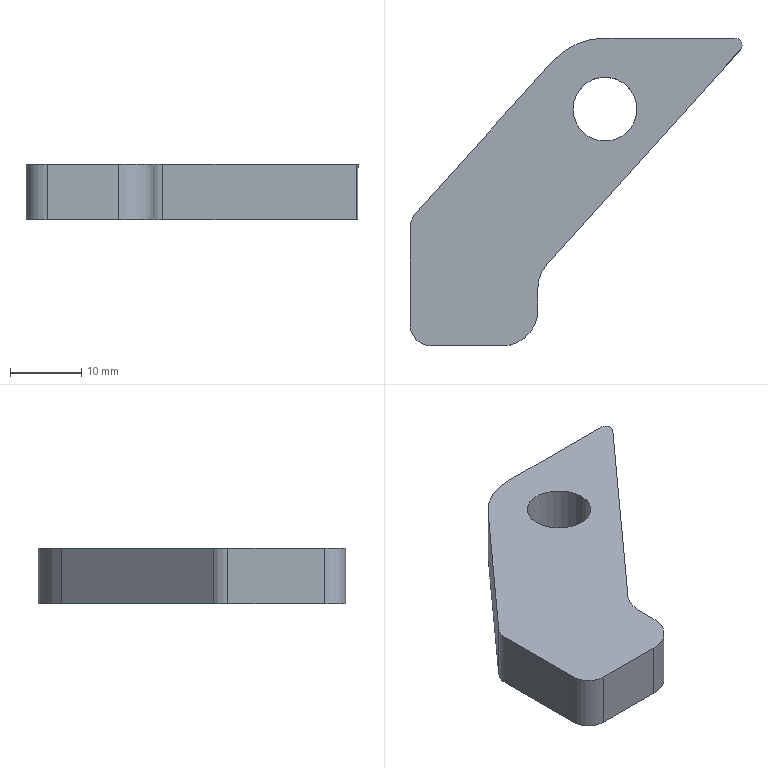Part | STEP file | 1 solid | 16 faces | box 46.755 x 43.333 x 7.8 mm | volume 7112 mm3 | cylinder 8 | plane 8 | commonest cylinder face diameters 6 x2 9 x2 10 x2 2 x1 20 x1
STEP:
#1=CARTESIAN_POINT('',(0.,0.,0.));
#2=DIRECTION('',(0.,0.,1.));
#3=DIRECTION('',(1.,0.,0.));
#4=AXIS2_PLACEMENT_3D('',#1,#2,#3);
#5=CARTESIAN_POINT('',(13.954,35.,7.8));
#6=VERTEX_POINT('',#5);
#7=CARTESIAN_POINT('',(4.954,35.,7.8));
#8=VERTEX_POINT('',#7);
#9=CARTESIAN_POINT('',(9.454,35.,7.8));
#10=DIRECTION('',(0.,0.,1.));
#11=DIRECTION('',(1.,0.,0.));
#12=AXIS2_PLACEMENT_3D('',#9,#10,#11);
#13=CIRCLE('',#12,4.5);
#14=CARTESIAN_POINT('',(9.454,35.,7.8));
#15=DIRECTION('',(0.,0.,1.));
#16=DIRECTION('',(1.,0.,0.));
#17=AXIS2_PLACEMENT_3D('',#14,#15,#16);
#18=CYLINDRICAL_SURFACE('',#17,4.5);
#19=CARTESIAN_POINT('',(0.,0.));
#20=DIRECTION('',(1.,0.));
#21=VECTOR('',#20,1.);
#22=LINE('',#19,#21);
#23=(GEOMETRIC_REPRESENTATION_CONTEXT(2)PARAMETRIC_REPRESENTATION_CONTEXT()REPRESENTATION_CONTEXT('',''));
#24=DEFINITIONAL_REPRESENTATION('',(#22),#23);
#25=PCURVE('',#18,#24);
#26=CARTESIAN_POINT('',(-15.,4.667,7.8));
#27=DIRECTION('',(0.,0.,-1.));
#28=DIRECTION('',(-1.,0.,0.));
#29=AXIS2_PLACEMENT_3D('',#26,#27,#28);
#30=PLANE('',#29);
#31=CARTESIAN_POINT('',(-28.954,30.333));
#32=CARTESIAN_POINT('',(-28.954,38.128));
#33=CARTESIAN_POINT('',(-22.204,34.23));
#34=CARTESIAN_POINT('',(-15.454,30.333));
#35=CARTESIAN_POINT('',(-22.204,26.436));
#36=CARTESIAN_POINT('',(-28.954,22.539));
#37=CARTESIAN_POINT('',(-28.954,30.333));
#38=(BOUNDED_CURVE()B_SPLINE_CURVE(2,(#31,#32,#33,#34,#35,#36,#37),.UNSPECIFIED.,.T.,.F.)B_SPLINE_CURVE_WITH_KNOTS((1,2,2,2,2,1),(-2.094,0.,2.094,4.189,6.283,8.378),.UNSPECIFIED.)CURVE()GEOMETRIC_REPRESENTATION_ITEM()RATIONAL_B_SPLINE_CURVE((1.,0.5,1.,0.5,1.,0.5,1.))REPRESENTATION_ITEM(''));
#39=(GEOMETRIC_REPRESENTATION_CONTEXT(2)PARAMETRIC_REPRESENTATION_CONTEXT()REPRESENTATION_CONTEXT('',''));
#40=DEFINITIONAL_REPRESENTATION('',(#38),#39);
#41=PCURVE('',#30,#40);
#42=SURFACE_CURVE('',#13,(#25,#41),.PCURVE_S1.);
#43=EDGE_CURVE('',#6,#8,#42,.T.);
#44=ORIENTED_EDGE('',*,*,#43,.F.);
#45=CARTESIAN_POINT('',(13.954,35.,0.));
#46=VERTEX_POINT('',#45);
#47=CARTESIAN_POINT('',(13.954,35.,7.8));
#48=DIRECTION('',(0.,0.,1.));
#49=VECTOR('',#48,1.);
#50=LINE('',#47,#49);
#51=CARTESIAN_POINT('',(0.,0.));
#52=DIRECTION('',(0.,1.));
#53=VECTOR('',#52,1.);
#54=LINE('',#51,#53);
#55=(GEOMETRIC_REPRESENTATION_CONTEXT(2)PARAMETRIC_REPRESENTATION_CONTEXT()REPRESENTATION_CONTEXT('',''));
#56=DEFINITIONAL_REPRESENTATION('',(#54),#55);
#57=PCURVE('',#18,#56);
#58=CARTESIAN_POINT('',(9.454,35.,7.8));
#59=DIRECTION('',(0.,0.,1.));
#60=DIRECTION('',(1.,0.,0.));
#61=AXIS2_PLACEMENT_3D('',#58,#59,#60);
#62=CYLINDRICAL_SURFACE('',#61,4.5);
#63=CARTESIAN_POINT('',(6.283,0.));
#64=DIRECTION('',(0.,1.));
#65=VECTOR('',#64,1.);
#66=LINE('',#63,#65);
#67=(GEOMETRIC_REPRESENTATION_CONTEXT(2)PARAMETRIC_REPRESENTATION_CONTEXT()REPRESENTATION_CONTEXT('',''));
#68=DEFINITIONAL_REPRESENTATION('',(#66),#67);
#69=PCURVE('',#62,#68);
#70=SURFACE_CURVE('',#50,(#57,#69),.PCURVE_S1.);
#71=EDGE_CURVE('',#46,#6,#70,.T.);
#72=ORIENTED_EDGE('',*,*,#71,.F.);
#73=CARTESIAN_POINT('',(4.954,35.,0.));
#74=VERTEX_POINT('',#73);
#75=CARTESIAN_POINT('',(9.454,35.,0.));
#76=DIRECTION('',(0.,0.,-1.));
#77=DIRECTION('',(-1.,0.,0.));
#78=AXIS2_PLACEMENT_3D('',#75,#76,#77);
#79=CIRCLE('',#78,4.5);
#80=CARTESIAN_POINT('',(3.142,-7.8));
#81=DIRECTION('',(-1.,0.));
#82=VECTOR('',#81,1.);
#83=LINE('',#80,#82);
#84=(GEOMETRIC_REPRESENTATION_CONTEXT(2)PARAMETRIC_REPRESENTATION_CONTEXT()REPRESENTATION_CONTEXT('',''));
#85=DEFINITIONAL_REPRESENTATION('',(#83),#84);
#86=PCURVE('',#18,#85);
#87=CARTESIAN_POINT('',(-15.,4.667,0.));
#88=DIRECTION('',(0.,0.,-1.));
#89=DIRECTION('',(-1.,0.,0.));
#90=AXIS2_PLACEMENT_3D('',#87,#88,#89);
#91=PLANE('',#90);
#92=CARTESIAN_POINT('',(-24.454,30.333));
#93=DIRECTION('',(1.,0.));
#94=AXIS2_PLACEMENT_2D('',#92,#93);
#95=CIRCLE('',#94,4.5);
#96=(GEOMETRIC_REPRESENTATION_CONTEXT(2)PARAMETRIC_REPRESENTATION_CONTEXT()REPRESENTATION_CONTEXT('',''));
#97=DEFINITIONAL_REPRESENTATION('',(#95),#96);
#98=PCURVE('',#91,#97);
#99=SURFACE_CURVE('',#79,(#86,#98),.PCURVE_S1.);
#100=EDGE_CURVE('',#74,#46,#99,.T.);
#101=ORIENTED_EDGE('',*,*,#100,.F.);
#102=CARTESIAN_POINT('',(4.954,35.,7.8));
#103=DIRECTION('',(0.,0.,1.));
#104=VECTOR('',#103,1.);
#105=LINE('',#102,#104);
#106=CARTESIAN_POINT('',(3.142,0.));
#107=DIRECTION('',(0.,1.));
#108=VECTOR('',#107,1.);
#109=LINE('',#106,#108);
#110=(GEOMETRIC_REPRESENTATION_CONTEXT(2)PARAMETRIC_REPRESENTATION_CONTEXT()REPRESENTATION_CONTEXT('',''));
#111=DEFINITIONAL_REPRESENTATION('',(#109),#110);
#112=PCURVE('',#18,#111);
#113=CARTESIAN_POINT('',(3.142,0.));
#114=DIRECTION('',(0.,1.));
#115=VECTOR('',#114,1.);
#116=LINE('',#113,#115);
#117=(GEOMETRIC_REPRESENTATION_CONTEXT(2)PARAMETRIC_REPRESENTATION_CONTEXT()REPRESENTATION_CONTEXT('',''));
#118=DEFINITIONAL_REPRESENTATION('',(#116),#117);
#119=PCURVE('',#62,#118);
#120=SURFACE_CURVE('',#105,(#112,#119),.PCURVE_S1.);
#121=EDGE_CURVE('',#74,#8,#120,.T.);
#122=ORIENTED_EDGE('',*,*,#121,.T.);
#123=EDGE_LOOP('',(#44,#72,#101,#122));
#124=FACE_BOUND('',#123,.F.);
#125=ADVANCED_FACE('',(#124),#18,.F.);
#126=CARTESIAN_POINT('',(9.454,35.,0.));
#127=DIRECTION('',(0.,0.,-1.));
#128=DIRECTION('',(-1.,0.,0.));
#129=AXIS2_PLACEMENT_3D('',#126,#127,#128);
#130=CIRCLE('',#129,4.5);
#131=CARTESIAN_POINT('',(-24.454,30.333));
#132=DIRECTION('',(1.,0.));
#133=AXIS2_PLACEMENT_2D('',#131,#132);
#134=CIRCLE('',#133,4.5);
#135=(GEOMETRIC_REPRESENTATION_CONTEXT(2)PARAMETRIC_REPRESENTATION_CONTEXT()REPRESENTATION_CONTEXT('',''));
#136=DEFINITIONAL_REPRESENTATION('',(#134),#135);
#137=PCURVE('',#91,#136);
#138=CARTESIAN_POINT('',(9.425,-7.8));
#139=DIRECTION('',(-1.,0.));
#140=VECTOR('',#139,1.);
#141=LINE('',#138,#140);
#142=(GEOMETRIC_REPRESENTATION_CONTEXT(2)PARAMETRIC_REPRESENTATION_CONTEXT()REPRESENTATION_CONTEXT('',''));
#143=DEFINITIONAL_REPRESENTATION('',(#141),#142);
#144=PCURVE('',#62,#143);
#145=SURFACE_CURVE('',#130,(#137,#144),.PCURVE_S1.);
#146=EDGE_CURVE('',#46,#74,#145,.T.);
#147=ORIENTED_EDGE('',*,*,#146,.F.);
#148=ORIENTED_EDGE('',*,*,#100,.F.);
#149=EDGE_LOOP('',(#147,#148));
#150=FACE_BOUND('',#149,.T.);
#151=CARTESIAN_POINT('',(-18.,4.667,0.));
#152=VERTEX_POINT('',#151);
#153=CARTESIAN_POINT('',(-15.,1.667,0.));
#154=VERTEX_POINT('',#153);
#155=CARTESIAN_POINT('',(-15.,4.667,0.));
#156=DIRECTION('',(0.,0.,1.));
#157=DIRECTION('',(-1.,0.,0.));
#158=AXIS2_PLACEMENT_3D('',#155,#156,#157);
#159=CIRCLE('',#158,3.);
#160=CARTESIAN_POINT('',(3.,0.));
#161=CARTESIAN_POINT('',(3.,-5.196));
#162=CARTESIAN_POINT('',(-1.5,-2.598));
#163=CARTESIAN_POINT('',(-6.,0.));
#164=CARTESIAN_POINT('',(-1.5,2.598));
#165=CARTESIAN_POINT('',(3.,5.196));
#166=CARTESIAN_POINT('',(3.,0.));
#167=(BOUNDED_CURVE()B_SPLINE_CURVE(2,(#160,#161,#162,#163,#164,#165,#166),.UNSPECIFIED.,.T.,.F.)B_SPLINE_CURVE_WITH_KNOTS((1,2,2,2,2,1),(-2.094,0.,2.094,4.189,6.283,8.378),.UNSPECIFIED.)CURVE()GEOMETRIC_REPRESENTATION_ITEM()RATIONAL_B_SPLINE_CURVE((1.,0.5,1.,0.5,1.,0.5,1.))REPRESENTATION_ITEM(''));
#168=(GEOMETRIC_REPRESENTATION_CONTEXT(2)PARAMETRIC_REPRESENTATION_CONTEXT()REPRESENTATION_CONTEXT('',''));
#169=DEFINITIONAL_REPRESENTATION('',(#167),#168);
#170=PCURVE('',#91,#169);
#171=CARTESIAN_POINT('',(-15.,4.667,7.8));
#172=DIRECTION('',(0.,0.,-1.));
#173=DIRECTION('',(-1.,0.,0.));
#174=AXIS2_PLACEMENT_3D('',#171,#172,#173);
#175=CYLINDRICAL_SURFACE('',#174,3.);
#176=CARTESIAN_POINT('',(6.283,7.8));
#177=DIRECTION('',(-1.,0.));
#178=VECTOR('',#177,1.);
#179=LINE('',#176,#178);
#180=(GEOMETRIC_REPRESENTATION_CONTEXT(2)PARAMETRIC_REPRESENTATION_CONTEXT()REPRESENTATION_CONTEXT('',''));
#181=DEFINITIONAL_REPRESENTATION('',(#179),#180);
#182=PCURVE('',#175,#181);
#183=SURFACE_CURVE('',#159,(#170,#182),.PCURVE_S1.);
#184=EDGE_CURVE('',#152,#154,#183,.T.);
#185=ORIENTED_EDGE('',*,*,#184,.F.);
#186=CARTESIAN_POINT('',(-18.,18.293,0.));
#187=VERTEX_POINT('',#186);
#188=CARTESIAN_POINT('',(-18.,4.667,0.));
#189=DIRECTION('',(0.,-1.,0.));
#190=VECTOR('',#189,1.);
#191=LINE('',#188,#190);
#192=CARTESIAN_POINT('',(3.,0.));
#193=DIRECTION('',(0.,-1.));
#194=VECTOR('',#193,1.);
#195=LINE('',#192,#194);
#196=(GEOMETRIC_REPRESENTATION_CONTEXT(2)PARAMETRIC_REPRESENTATION_CONTEXT()REPRESENTATION_CONTEXT('',''));
#197=DEFINITIONAL_REPRESENTATION('',(#195),#196);
#198=PCURVE('',#91,#197);
#199=CARTESIAN_POINT('',(-18.,4.667,7.8));
#200=DIRECTION('',(1.,0.,0.));
#201=DIRECTION('',(0.,0.,1.));
#202=AXIS2_PLACEMENT_3D('',#199,#200,#201);
#203=PLANE('',#202);
#204=CARTESIAN_POINT('',(-7.8,0.));
#205=DIRECTION('',(0.,1.));
#206=VECTOR('',#205,1.);
#207=LINE('',#204,#206);
#208=(GEOMETRIC_REPRESENTATION_CONTEXT(2)PARAMETRIC_REPRESENTATION_CONTEXT()REPRESENTATION_CONTEXT('',''));
#209=DEFINITIONAL_REPRESENTATION('',(#207),#208);
#210=PCURVE('',#203,#209);
#211=SURFACE_CURVE('',#191,(#198,#210),.PCURVE_S1.);
#212=EDGE_CURVE('',#187,#152,#211,.T.);
#213=ORIENTED_EDGE('',*,*,#212,.F.);
#214=CARTESIAN_POINT('',(-17.23,20.3,0.));
#215=VERTEX_POINT('',#214);
#216=CARTESIAN_POINT('',(-15.,18.293,0.));
#217=DIRECTION('',(0.,0.,1.));
#218=DIRECTION('',(1.,0.,0.));
#219=AXIS2_PLACEMENT_3D('',#216,#217,#218);
#220=CIRCLE('',#219,3.);
#221=CARTESIAN_POINT('',(-3.,13.627));
#222=CARTESIAN_POINT('',(-3.,18.823));
#223=CARTESIAN_POINT('',(1.5,16.225));
#224=CARTESIAN_POINT('',(6.,13.627));
#225=CARTESIAN_POINT('',(1.5,11.028));
#226=CARTESIAN_POINT('',(-3.,8.43));
#227=CARTESIAN_POINT('',(-3.,13.627));
#228=(BOUNDED_CURVE()B_SPLINE_CURVE(2,(#221,#222,#223,#224,#225,#226,#227),.UNSPECIFIED.,.T.,.F.)B_SPLINE_CURVE_WITH_KNOTS((1,2,2,2,2,1),(-2.094,0.,2.094,4.189,6.283,8.378),.UNSPECIFIED.)CURVE()GEOMETRIC_REPRESENTATION_ITEM()RATIONAL_B_SPLINE_CURVE((1.,0.5,1.,0.5,1.,0.5,1.))REPRESENTATION_ITEM(''));
#229=(GEOMETRIC_REPRESENTATION_CONTEXT(2)PARAMETRIC_REPRESENTATION_CONTEXT()REPRESENTATION_CONTEXT('',''));
#230=DEFINITIONAL_REPRESENTATION('',(#228),#229);
#231=PCURVE('',#91,#230);
#232=CARTESIAN_POINT('',(-15.,18.293,7.8));
#233=DIRECTION('',(0.,0.,-1.));
#234=DIRECTION('',(-1.,0.,0.));
#235=AXIS2_PLACEMENT_3D('',#232,#233,#234);
#236=CYLINDRICAL_SURFACE('',#235,3.);
#237=CARTESIAN_POINT('',(3.142,7.8));
#238=DIRECTION('',(-1.,0.));
#239=VECTOR('',#238,1.);
#240=LINE('',#237,#239);
#241=(GEOMETRIC_REPRESENTATION_CONTEXT(2)PARAMETRIC_REPRESENTATION_CONTEXT()REPRESENTATION_CONTEXT('',''));
#242=DEFINITIONAL_REPRESENTATION('',(#240),#241);
#243=PCURVE('',#236,#242);
#244=SURFACE_CURVE('',#220,(#231,#243),.PCURVE_S1.);
#245=EDGE_CURVE('',#215,#187,#244,.T.);
#246=ORIENTED_EDGE('',*,*,#245,.F.);
#247=CARTESIAN_POINT('',(2.021,41.69,0.));
#248=VERTEX_POINT('',#247);
#249=CARTESIAN_POINT('',(-17.23,20.3,0.));
#250=DIRECTION('',(-0.669,-0.7433,0.));
#251=VECTOR('',#250,1.);
#252=LINE('',#249,#251);
#253=CARTESIAN_POINT('',(2.23,15.633));
#254=DIRECTION('',(0.669,-0.7433));
#255=VECTOR('',#254,1.);
#256=LINE('',#253,#255);
#257=(GEOMETRIC_REPRESENTATION_CONTEXT(2)PARAMETRIC_REPRESENTATION_CONTEXT()REPRESENTATION_CONTEXT('',''));
#258=DEFINITIONAL_REPRESENTATION('',(#256),#257);
#259=PCURVE('',#91,#258);
#260=CARTESIAN_POINT('',(-17.23,20.3,7.8));
#261=DIRECTION('',(0.7433,-0.669,0.));
#262=DIRECTION('',(0.,0.,-1.));
#263=AXIS2_PLACEMENT_3D('',#260,#261,#262);
#264=PLANE('',#263);
#265=CARTESIAN_POINT('',(7.8,0.));
#266=DIRECTION('',(0.,-1.));
#267=VECTOR('',#266,1.);
#268=LINE('',#265,#267);
#269=(GEOMETRIC_REPRESENTATION_CONTEXT(2)PARAMETRIC_REPRESENTATION_CONTEXT()REPRESENTATION_CONTEXT('',''));
#270=DEFINITIONAL_REPRESENTATION('',(#268),#269);
#271=PCURVE('',#264,#270);
#272=SURFACE_CURVE('',#252,(#259,#271),.PCURVE_S1.);
#273=EDGE_CURVE('',#248,#215,#272,.T.);
#274=ORIENTED_EDGE('',*,*,#273,.F.);
#275=CARTESIAN_POINT('',(9.454,45.,0.));
#276=VERTEX_POINT('',#275);
#277=CARTESIAN_POINT('',(9.454,35.,0.));
#278=DIRECTION('',(0.,0.,1.));
#279=DIRECTION('',(-1.,0.,0.));
#280=AXIS2_PLACEMENT_3D('',#277,#278,#279);
#281=CIRCLE('',#280,10.);
#282=CARTESIAN_POINT('',(-14.454,30.333));
#283=CARTESIAN_POINT('',(-14.454,13.013));
#284=CARTESIAN_POINT('',(-29.454,21.673));
#285=CARTESIAN_POINT('',(-44.454,30.333));
#286=CARTESIAN_POINT('',(-29.454,38.994));
#287=CARTESIAN_POINT('',(-14.454,47.654));
#288=CARTESIAN_POINT('',(-14.454,30.333));
#289=(BOUNDED_CURVE()B_SPLINE_CURVE(2,(#282,#283,#284,#285,#286,#287,#288),.UNSPECIFIED.,.T.,.F.)B_SPLINE_CURVE_WITH_KNOTS((1,2,2,2,2,1),(-2.094,0.,2.094,4.189,6.283,8.378),.UNSPECIFIED.)CURVE()GEOMETRIC_REPRESENTATION_ITEM()RATIONAL_B_SPLINE_CURVE((1.,0.5,1.,0.5,1.,0.5,1.))REPRESENTATION_ITEM(''));
#290=(GEOMETRIC_REPRESENTATION_CONTEXT(2)PARAMETRIC_REPRESENTATION_CONTEXT()REPRESENTATION_CONTEXT('',''));
#291=DEFINITIONAL_REPRESENTATION('',(#289),#290);
#292=PCURVE('',#91,#291);
#293=CARTESIAN_POINT('',(9.454,35.,7.8));
#294=DIRECTION('',(0.,0.,-1.));
#295=DIRECTION('',(-1.,0.,0.));
#296=AXIS2_PLACEMENT_3D('',#293,#294,#295);
#297=CYLINDRICAL_SURFACE('',#296,10.);
#298=CARTESIAN_POINT('',(6.283,7.8));
#299=DIRECTION('',(-1.,0.));
#300=VECTOR('',#299,1.);
#301=LINE('',#298,#300);
#302=(GEOMETRIC_REPRESENTATION_CONTEXT(2)PARAMETRIC_REPRESENTATION_CONTEXT()REPRESENTATION_CONTEXT('',''));
#303=DEFINITIONAL_REPRESENTATION('',(#301),#302);
#304=PCURVE('',#297,#303);
#305=SURFACE_CURVE('',#281,(#292,#304),.PCURVE_S1.);
#306=EDGE_CURVE('',#276,#248,#305,.T.);
#307=ORIENTED_EDGE('',*,*,#306,.F.);
#308=CARTESIAN_POINT('',(27.755,45.,0.));
#309=VERTEX_POINT('',#308);
#310=CARTESIAN_POINT('',(9.454,45.,0.));
#311=DIRECTION('',(-1.,0.,0.));
#312=VECTOR('',#311,1.);
#313=LINE('',#310,#312);
#314=CARTESIAN_POINT('',(-24.454,40.333));
#315=DIRECTION('',(1.,0.));
#316=VECTOR('',#315,1.);
#317=LINE('',#314,#316);
#318=(GEOMETRIC_REPRESENTATION_CONTEXT(2)PARAMETRIC_REPRESENTATION_CONTEXT()REPRESENTATION_CONTEXT('',''));
#319=DEFINITIONAL_REPRESENTATION('',(#317),#318);
#320=PCURVE('',#91,#319);
#321=CARTESIAN_POINT('',(9.454,45.,7.8));
#322=DIRECTION('',(0.,-1.,0.));
#323=DIRECTION('',(0.,0.,-1.));
#324=AXIS2_PLACEMENT_3D('',#321,#322,#323);
#325=PLANE('',#324);
#326=CARTESIAN_POINT('',(7.8,0.));
#327=DIRECTION('',(0.,-1.));
#328=VECTOR('',#327,1.);
#329=LINE('',#326,#328);
#330=(GEOMETRIC_REPRESENTATION_CONTEXT(2)PARAMETRIC_REPRESENTATION_CONTEXT()REPRESENTATION_CONTEXT('',''));
#331=DEFINITIONAL_REPRESENTATION('',(#329),#330);
#332=PCURVE('',#325,#331);
#333=SURFACE_CURVE('',#313,(#320,#332),.PCURVE_S1.);
#334=EDGE_CURVE('',#309,#276,#333,.T.);
#335=ORIENTED_EDGE('',*,*,#334,.F.);
#336=CARTESIAN_POINT('',(28.498,43.331,0.));
#337=VERTEX_POINT('',#336);
#338=CARTESIAN_POINT('',(27.755,44.,0.));
#339=DIRECTION('',(0.,0.,1.));
#340=DIRECTION('',(-1.,0.,0.));
#341=AXIS2_PLACEMENT_3D('',#338,#339,#340);
#342=CIRCLE('',#341,1.);
#343=CARTESIAN_POINT('',(-41.755,39.333));
#344=CARTESIAN_POINT('',(-41.755,37.601));
#345=CARTESIAN_POINT('',(-43.255,38.467));
#346=CARTESIAN_POINT('',(-44.755,39.333));
#347=CARTESIAN_POINT('',(-43.255,40.199));
#348=CARTESIAN_POINT('',(-41.755,41.065));
#349=CARTESIAN_POINT('',(-41.755,39.333));
#350=(BOUNDED_CURVE()B_SPLINE_CURVE(2,(#343,#344,#345,#346,#347,#348,#349),.UNSPECIFIED.,.T.,.F.)B_SPLINE_CURVE_WITH_KNOTS((1,2,2,2,2,1),(-2.094,0.,2.094,4.189,6.283,8.378),.UNSPECIFIED.)CURVE()GEOMETRIC_REPRESENTATION_ITEM()RATIONAL_B_SPLINE_CURVE((1.,0.5,1.,0.5,1.,0.5,1.))REPRESENTATION_ITEM(''));
#351=(GEOMETRIC_REPRESENTATION_CONTEXT(2)PARAMETRIC_REPRESENTATION_CONTEXT()REPRESENTATION_CONTEXT('',''));
#352=DEFINITIONAL_REPRESENTATION('',(#350),#351);
#353=PCURVE('',#91,#352);
#354=CARTESIAN_POINT('',(27.755,44.,7.8));
#355=DIRECTION('',(0.,0.,-1.));
#356=DIRECTION('',(-1.,0.,0.));
#357=AXIS2_PLACEMENT_3D('',#354,#355,#356);
#358=CYLINDRICAL_SURFACE('',#357,1.);
#359=CARTESIAN_POINT('',(6.283,7.8));
#360=DIRECTION('',(-1.,0.));
#361=VECTOR('',#360,1.);
#362=LINE('',#359,#361);
#363=(GEOMETRIC_REPRESENTATION_CONTEXT(2)PARAMETRIC_REPRESENTATION_CONTEXT()REPRESENTATION_CONTEXT('',''));
#364=DEFINITIONAL_REPRESENTATION('',(#362),#363);
#365=PCURVE('',#358,#364);
#366=SURFACE_CURVE('',#342,(#353,#365),.PCURVE_S1.);
#367=EDGE_CURVE('',#337,#309,#366,.T.);
#368=ORIENTED_EDGE('',*,*,#367,.F.);
#369=CARTESIAN_POINT('',(1.284,13.093,0.));
#370=VERTEX_POINT('',#369);
#371=CARTESIAN_POINT('',(28.498,43.331,0.));
#372=DIRECTION('',(0.669,0.7433,0.));
#373=VECTOR('',#372,1.);
#374=LINE('',#371,#373);
#375=CARTESIAN_POINT('',(-43.498,38.664));
#376=DIRECTION('',(-0.669,0.7433));
#377=VECTOR('',#376,1.);
#378=LINE('',#375,#377);
#379=(GEOMETRIC_REPRESENTATION_CONTEXT(2)PARAMETRIC_REPRESENTATION_CONTEXT()REPRESENTATION_CONTEXT('',''));
#380=DEFINITIONAL_REPRESENTATION('',(#378),#379);
#381=PCURVE('',#91,#380);
#382=CARTESIAN_POINT('',(28.498,43.331,7.8));
#383=DIRECTION('',(-0.7433,0.669,0.));
#384=DIRECTION('',(0.,0.,1.));
#385=AXIS2_PLACEMENT_3D('',#382,#383,#384);
#386=PLANE('',#385);
#387=CARTESIAN_POINT('',(-7.8,0.));
#388=DIRECTION('',(0.,1.));
#389=VECTOR('',#388,1.);
#390=LINE('',#387,#389);
#391=(GEOMETRIC_REPRESENTATION_CONTEXT(2)PARAMETRIC_REPRESENTATION_CONTEXT()REPRESENTATION_CONTEXT('',''));
#392=DEFINITIONAL_REPRESENTATION('',(#390),#391);
#393=PCURVE('',#386,#392);
#394=SURFACE_CURVE('',#374,(#381,#393),.PCURVE_S1.);
#395=EDGE_CURVE('',#370,#337,#394,.T.);
#396=ORIENTED_EDGE('',*,*,#395,.F.);
#397=CARTESIAN_POINT('',(0.,9.748,0.));
#398=VERTEX_POINT('',#397);
#399=CARTESIAN_POINT('',(5.,9.748,0.));
#400=DIRECTION('',(0.,0.,-1.));
#401=DIRECTION('',(1.,0.,0.));
#402=AXIS2_PLACEMENT_3D('',#399,#400,#401);
#403=CIRCLE('',#402,5.);
#404=CARTESIAN_POINT('',(-20.,5.081));
#405=DIRECTION('',(-1.,0.));
#406=AXIS2_PLACEMENT_2D('',#404,#405);
#407=CIRCLE('',#406,5.);
#408=(GEOMETRIC_REPRESENTATION_CONTEXT(2)PARAMETRIC_REPRESENTATION_CONTEXT()REPRESENTATION_CONTEXT('',''));
#409=DEFINITIONAL_REPRESENTATION('',(#407),#408);
#410=PCURVE('',#91,#409);
#411=CARTESIAN_POINT('',(5.,9.748,7.8));
#412=DIRECTION('',(0.,0.,-1.));
#413=DIRECTION('',(-1.,0.,0.));
#414=AXIS2_PLACEMENT_3D('',#411,#412,#413);
#415=CYLINDRICAL_SURFACE('',#414,5.);
#416=CARTESIAN_POINT('',(-3.142,7.8));
#417=DIRECTION('',(1.,0.));
#418=VECTOR('',#417,1.);
#419=LINE('',#416,#418);
#420=(GEOMETRIC_REPRESENTATION_CONTEXT(2)PARAMETRIC_REPRESENTATION_CONTEXT()REPRESENTATION_CONTEXT('',''));
#421=DEFINITIONAL_REPRESENTATION('',(#419),#420);
#422=PCURVE('',#415,#421);
#423=SURFACE_CURVE('',#403,(#410,#422),.PCURVE_S1.);
#424=EDGE_CURVE('',#398,#370,#423,.T.);
#425=ORIENTED_EDGE('',*,*,#424,.F.);
#426=CARTESIAN_POINT('',(0.,6.667,0.));
#427=VERTEX_POINT('',#426);
#428=CARTESIAN_POINT('',(0.,9.748,0.));
#429=DIRECTION('',(0.,1.,0.));
#430=VECTOR('',#429,1.);
#431=LINE('',#428,#430);
#432=CARTESIAN_POINT('',(-15.,5.081));
#433=DIRECTION('',(0.,1.));
#434=VECTOR('',#433,1.);
#435=LINE('',#432,#434);
#436=(GEOMETRIC_REPRESENTATION_CONTEXT(2)PARAMETRIC_REPRESENTATION_CONTEXT()REPRESENTATION_CONTEXT('',''));
#437=DEFINITIONAL_REPRESENTATION('',(#435),#436);
#438=PCURVE('',#91,#437);
#439=CARTESIAN_POINT('',(0.,9.748,7.8));
#440=DIRECTION('',(-1.,0.,0.));
#441=DIRECTION('',(0.,1.,0.));
#442=AXIS2_PLACEMENT_3D('',#439,#440,#441);
#443=PLANE('',#442);
#444=CARTESIAN_POINT('',(0.,7.8));
#445=DIRECTION('',(1.,0.));
#446=VECTOR('',#445,1.);
#447=LINE('',#444,#446);
#448=(GEOMETRIC_REPRESENTATION_CONTEXT(2)PARAMETRIC_REPRESENTATION_CONTEXT()REPRESENTATION_CONTEXT('',''));
#449=DEFINITIONAL_REPRESENTATION('',(#447),#448);
#450=PCURVE('',#443,#449);
#451=SURFACE_CURVE('',#431,(#438,#450),.PCURVE_S1.);
#452=EDGE_CURVE('',#427,#398,#451,.T.);
#453=ORIENTED_EDGE('',*,*,#452,.F.);
#454=CARTESIAN_POINT('',(-5.,1.667,0.));
#455=VERTEX_POINT('',#454);
#456=CARTESIAN_POINT('',(-5.,6.667,0.));
#457=DIRECTION('',(0.,0.,1.));
#458=DIRECTION('',(-1.,0.,0.));
#459=AXIS2_PLACEMENT_3D('',#456,#457,#458);
#460=CIRCLE('',#459,5.);
#461=CARTESIAN_POINT('',(-5.,2.));
#462=CARTESIAN_POINT('',(-5.,-6.66));
#463=CARTESIAN_POINT('',(-12.5,-2.33));
#464=CARTESIAN_POINT('',(-20.,2.));
#465=CARTESIAN_POINT('',(-12.5,6.33));
#466=CARTESIAN_POINT('',(-5.,10.66));
#467=CARTESIAN_POINT('',(-5.,2.));
#468=(BOUNDED_CURVE()B_SPLINE_CURVE(2,(#461,#462,#463,#464,#465,#466,#467),.UNSPECIFIED.,.T.,.F.)B_SPLINE_CURVE_WITH_KNOTS((1,2,2,2,2,1),(-2.094,0.,2.094,4.189,6.283,8.378),.UNSPECIFIED.)CURVE()GEOMETRIC_REPRESENTATION_ITEM()RATIONAL_B_SPLINE_CURVE((1.,0.5,1.,0.5,1.,0.5,1.))REPRESENTATION_ITEM(''));
#469=(GEOMETRIC_REPRESENTATION_CONTEXT(2)PARAMETRIC_REPRESENTATION_CONTEXT()REPRESENTATION_CONTEXT('',''));
#470=DEFINITIONAL_REPRESENTATION('',(#468),#469);
#471=PCURVE('',#91,#470);
#472=CARTESIAN_POINT('',(-5.,6.667,7.8));
#473=DIRECTION('',(0.,0.,-1.));
#474=DIRECTION('',(-1.,0.,0.));
#475=AXIS2_PLACEMENT_3D('',#472,#473,#474);
#476=CYLINDRICAL_SURFACE('',#475,5.);
#477=CARTESIAN_POINT('',(6.283,7.8));
#478=DIRECTION('',(-1.,0.));
#479=VECTOR('',#478,1.);
#480=LINE('',#477,#479);
#481=(GEOMETRIC_REPRESENTATION_CONTEXT(2)PARAMETRIC_REPRESENTATION_CONTEXT()REPRESENTATION_CONTEXT('',''));
#482=DEFINITIONAL_REPRESENTATION('',(#480),#481);
#483=PCURVE('',#476,#482);
#484=SURFACE_CURVE('',#460,(#471,#483),.PCURVE_S1.);
#485=EDGE_CURVE('',#455,#427,#484,.T.);
#486=ORIENTED_EDGE('',*,*,#485,.F.);
#487=CARTESIAN_POINT('',(-5.,1.667,0.));
#488=DIRECTION('',(1.,0.,0.));
#489=VECTOR('',#488,1.);
#490=LINE('',#487,#489);
#491=CARTESIAN_POINT('',(-10.,-3.));
#492=DIRECTION('',(-1.,0.));
#493=VECTOR('',#492,1.);
#494=LINE('',#491,#493);
#495=(GEOMETRIC_REPRESENTATION_CONTEXT(2)PARAMETRIC_REPRESENTATION_CONTEXT()REPRESENTATION_CONTEXT('',''));
#496=DEFINITIONAL_REPRESENTATION('',(#494),#495);
#497=PCURVE('',#91,#496);
#498=CARTESIAN_POINT('',(-5.,1.667,7.8));
#499=DIRECTION('',(0.,1.,0.));
#500=DIRECTION('',(1.,0.,0.));
#501=AXIS2_PLACEMENT_3D('',#498,#499,#500);
#502=PLANE('',#501);
#503=CARTESIAN_POINT('',(0.,7.8));
#504=DIRECTION('',(1.,0.));
#505=VECTOR('',#504,1.);
#506=LINE('',#503,#505);
#507=(GEOMETRIC_REPRESENTATION_CONTEXT(2)PARAMETRIC_REPRESENTATION_CONTEXT()REPRESENTATION_CONTEXT('',''));
#508=DEFINITIONAL_REPRESENTATION('',(#506),#507);
#509=PCURVE('',#502,#508);
#510=SURFACE_CURVE('',#490,(#497,#509),.PCURVE_S1.);
#511=EDGE_CURVE('',#154,#455,#510,.T.);
#512=ORIENTED_EDGE('',*,*,#511,.F.);
#513=EDGE_LOOP('',(#185,#213,#246,#274,#307,#335,#368,#396,#425,#453,#486,#512));
#514=FACE_BOUND('',#513,.T.);
#515=ADVANCED_FACE('',(#150,#514),#91,.T.);
#516=ORIENTED_EDGE('',*,*,#43,.F.);
#517=CARTESIAN_POINT('',(9.454,35.,7.8));
#518=DIRECTION('',(0.,0.,1.));
#519=DIRECTION('',(1.,0.,0.));
#520=AXIS2_PLACEMENT_3D('',#517,#518,#519);
#521=CIRCLE('',#520,4.5);
#522=CARTESIAN_POINT('',(-28.954,30.333));
#523=CARTESIAN_POINT('',(-28.954,38.128));
#524=CARTESIAN_POINT('',(-22.204,34.23));
#525=CARTESIAN_POINT('',(-15.454,30.333));
#526=CARTESIAN_POINT('',(-22.204,26.436));
#527=CARTESIAN_POINT('',(-28.954,22.539));
#528=CARTESIAN_POINT('',(-28.954,30.333));
#529=(BOUNDED_CURVE()B_SPLINE_CURVE(2,(#522,#523,#524,#525,#526,#527,#528),.UNSPECIFIED.,.T.,.F.)B_SPLINE_CURVE_WITH_KNOTS((1,2,2,2,2,1),(-2.094,0.,2.094,4.189,6.283,8.378),.UNSPECIFIED.)CURVE()GEOMETRIC_REPRESENTATION_ITEM()RATIONAL_B_SPLINE_CURVE((1.,0.5,1.,0.5,1.,0.5,1.))REPRESENTATION_ITEM(''));
#530=(GEOMETRIC_REPRESENTATION_CONTEXT(2)PARAMETRIC_REPRESENTATION_CONTEXT()REPRESENTATION_CONTEXT('',''));
#531=DEFINITIONAL_REPRESENTATION('',(#529),#530);
#532=PCURVE('',#30,#531);
#533=CARTESIAN_POINT('',(0.,0.));
#534=DIRECTION('',(1.,0.));
#535=VECTOR('',#534,1.);
#536=LINE('',#533,#535);
#537=(GEOMETRIC_REPRESENTATION_CONTEXT(2)PARAMETRIC_REPRESENTATION_CONTEXT()REPRESENTATION_CONTEXT('',''));
#538=DEFINITIONAL_REPRESENTATION('',(#536),#537);
#539=PCURVE('',#62,#538);
#540=SURFACE_CURVE('',#521,(#532,#539),.PCURVE_S1.);
#541=EDGE_CURVE('',#8,#6,#540,.T.);
#542=ORIENTED_EDGE('',*,*,#541,.F.);
#543=EDGE_LOOP('',(#516,#542));
#544=FACE_BOUND('',#543,.T.);
#545=CARTESIAN_POINT('',(-18.,4.667,7.8));
#546=VERTEX_POINT('',#545);
#547=CARTESIAN_POINT('',(-15.,1.667,7.8));
#548=VERTEX_POINT('',#547);
#549=CARTESIAN_POINT('',(-15.,4.667,7.8));
#550=DIRECTION('',(0.,0.,1.));
#551=DIRECTION('',(-1.,0.,0.));
#552=AXIS2_PLACEMENT_3D('',#549,#550,#551);
#553=CIRCLE('',#552,3.);
#554=CARTESIAN_POINT('',(3.,0.));
#555=CARTESIAN_POINT('',(3.,-5.196));
#556=CARTESIAN_POINT('',(-1.5,-2.598));
#557=CARTESIAN_POINT('',(-6.,0.));
#558=CARTESIAN_POINT('',(-1.5,2.598));
#559=CARTESIAN_POINT('',(3.,5.196));
#560=CARTESIAN_POINT('',(3.,0.));
#561=(BOUNDED_CURVE()B_SPLINE_CURVE(2,(#554,#555,#556,#557,#558,#559,#560),.UNSPECIFIED.,.T.,.F.)B_SPLINE_CURVE_WITH_KNOTS((1,2,2,2,2,1),(-2.094,0.,2.094,4.189,6.283,8.378),.UNSPECIFIED.)CURVE()GEOMETRIC_REPRESENTATION_ITEM()RATIONAL_B_SPLINE_CURVE((1.,0.5,1.,0.5,1.,0.5,1.))REPRESENTATION_ITEM(''));
#562=(GEOMETRIC_REPRESENTATION_CONTEXT(2)PARAMETRIC_REPRESENTATION_CONTEXT()REPRESENTATION_CONTEXT('',''));
#563=DEFINITIONAL_REPRESENTATION('',(#561),#562);
#564=PCURVE('',#30,#563);
#565=CARTESIAN_POINT('',(6.283,0.));
#566=DIRECTION('',(-1.,0.));
#567=VECTOR('',#566,1.);
#568=LINE('',#565,#567);
#569=(GEOMETRIC_REPRESENTATION_CONTEXT(2)PARAMETRIC_REPRESENTATION_CONTEXT()REPRESENTATION_CONTEXT('',''));
#570=DEFINITIONAL_REPRESENTATION('',(#568),#569);
#571=PCURVE('',#175,#570);
#572=SURFACE_CURVE('',#553,(#564,#571),.PCURVE_S1.);
#573=EDGE_CURVE('',#546,#548,#572,.T.);
#574=ORIENTED_EDGE('',*,*,#573,.T.);
#575=CARTESIAN_POINT('',(-5.,1.667,7.8));
#576=VERTEX_POINT('',#575);
#577=CARTESIAN_POINT('',(-5.,1.667,7.8));
#578=DIRECTION('',(1.,0.,0.));
#579=VECTOR('',#578,1.);
#580=LINE('',#577,#579);
#581=CARTESIAN_POINT('',(-10.,-3.));
#582=DIRECTION('',(-1.,0.));
#583=VECTOR('',#582,1.);
#584=LINE('',#581,#583);
#585=(GEOMETRIC_REPRESENTATION_CONTEXT(2)PARAMETRIC_REPRESENTATION_CONTEXT()REPRESENTATION_CONTEXT('',''));
#586=DEFINITIONAL_REPRESENTATION('',(#584),#585);
#587=PCURVE('',#30,#586);
#588=CARTESIAN_POINT('',(0.,0.));
#589=DIRECTION('',(1.,0.));
#590=VECTOR('',#589,1.);
#591=LINE('',#588,#590);
#592=(GEOMETRIC_REPRESENTATION_CONTEXT(2)PARAMETRIC_REPRESENTATION_CONTEXT()REPRESENTATION_CONTEXT('',''));
#593=DEFINITIONAL_REPRESENTATION('',(#591),#592);
#594=PCURVE('',#502,#593);
#595=SURFACE_CURVE('',#580,(#587,#594),.PCURVE_S1.);
#596=EDGE_CURVE('',#548,#576,#595,.T.);
#597=ORIENTED_EDGE('',*,*,#596,.T.);
#598=CARTESIAN_POINT('',(0.,6.667,7.8));
#599=VERTEX_POINT('',#598);
#600=CARTESIAN_POINT('',(-5.,6.667,7.8));
#601=DIRECTION('',(0.,0.,1.));
#602=DIRECTION('',(-1.,0.,0.));
#603=AXIS2_PLACEMENT_3D('',#600,#601,#602);
#604=CIRCLE('',#603,5.);
#605=CARTESIAN_POINT('',(-5.,2.));
#606=CARTESIAN_POINT('',(-5.,-6.66));
#607=CARTESIAN_POINT('',(-12.5,-2.33));
#608=CARTESIAN_POINT('',(-20.,2.));
#609=CARTESIAN_POINT('',(-12.5,6.33));
#610=CARTESIAN_POINT('',(-5.,10.66));
#611=CARTESIAN_POINT('',(-5.,2.));
#612=(BOUNDED_CURVE()B_SPLINE_CURVE(2,(#605,#606,#607,#608,#609,#610,#611),.UNSPECIFIED.,.T.,.F.)B_SPLINE_CURVE_WITH_KNOTS((1,2,2,2,2,1),(-2.094,0.,2.094,4.189,6.283,8.378),.UNSPECIFIED.)CURVE()GEOMETRIC_REPRESENTATION_ITEM()RATIONAL_B_SPLINE_CURVE((1.,0.5,1.,0.5,1.,0.5,1.))REPRESENTATION_ITEM(''));
#613=(GEOMETRIC_REPRESENTATION_CONTEXT(2)PARAMETRIC_REPRESENTATION_CONTEXT()REPRESENTATION_CONTEXT('',''));
#614=DEFINITIONAL_REPRESENTATION('',(#612),#613);
#615=PCURVE('',#30,#614);
#616=CARTESIAN_POINT('',(6.283,0.));
#617=DIRECTION('',(-1.,0.));
#618=VECTOR('',#617,1.);
#619=LINE('',#616,#618);
#620=(GEOMETRIC_REPRESENTATION_CONTEXT(2)PARAMETRIC_REPRESENTATION_CONTEXT()REPRESENTATION_CONTEXT('',''));
#621=DEFINITIONAL_REPRESENTATION('',(#619),#620);
#622=PCURVE('',#476,#621);
#623=SURFACE_CURVE('',#604,(#615,#622),.PCURVE_S1.);
#624=EDGE_CURVE('',#576,#599,#623,.T.);
#625=ORIENTED_EDGE('',*,*,#624,.T.);
#626=CARTESIAN_POINT('',(0.,9.748,7.8));
#627=VERTEX_POINT('',#626);
#628=CARTESIAN_POINT('',(0.,9.748,7.8));
#629=DIRECTION('',(0.,1.,0.));
#630=VECTOR('',#629,1.);
#631=LINE('',#628,#630);
#632=CARTESIAN_POINT('',(-15.,5.081));
#633=DIRECTION('',(0.,1.));
#634=VECTOR('',#633,1.);
#635=LINE('',#632,#634);
#636=(GEOMETRIC_REPRESENTATION_CONTEXT(2)PARAMETRIC_REPRESENTATION_CONTEXT()REPRESENTATION_CONTEXT('',''));
#637=DEFINITIONAL_REPRESENTATION('',(#635),#636);
#638=PCURVE('',#30,#637);
#639=CARTESIAN_POINT('',(0.,0.));
#640=DIRECTION('',(1.,0.));
#641=VECTOR('',#640,1.);
#642=LINE('',#639,#641);
#643=(GEOMETRIC_REPRESENTATION_CONTEXT(2)PARAMETRIC_REPRESENTATION_CONTEXT()REPRESENTATION_CONTEXT('',''));
#644=DEFINITIONAL_REPRESENTATION('',(#642),#643);
#645=PCURVE('',#443,#644);
#646=SURFACE_CURVE('',#631,(#638,#645),.PCURVE_S1.);
#647=EDGE_CURVE('',#599,#627,#646,.T.);
#648=ORIENTED_EDGE('',*,*,#647,.T.);
#649=CARTESIAN_POINT('',(1.284,13.093,7.8));
#650=VERTEX_POINT('',#649);
#651=CARTESIAN_POINT('',(5.,9.748,7.8));
#652=DIRECTION('',(0.,0.,-1.));
#653=DIRECTION('',(1.,0.,0.));
#654=AXIS2_PLACEMENT_3D('',#651,#652,#653);
#655=CIRCLE('',#654,5.);
#656=CARTESIAN_POINT('',(-20.,5.081));
#657=DIRECTION('',(-1.,0.));
#658=AXIS2_PLACEMENT_2D('',#656,#657);
#659=CIRCLE('',#658,5.);
#660=(GEOMETRIC_REPRESENTATION_CONTEXT(2)PARAMETRIC_REPRESENTATION_CONTEXT()REPRESENTATION_CONTEXT('',''));
#661=DEFINITIONAL_REPRESENTATION('',(#659),#660);
#662=PCURVE('',#30,#661);
#663=CARTESIAN_POINT('',(-3.142,0.));
#664=DIRECTION('',(1.,0.));
#665=VECTOR('',#664,1.);
#666=LINE('',#663,#665);
#667=(GEOMETRIC_REPRESENTATION_CONTEXT(2)PARAMETRIC_REPRESENTATION_CONTEXT()REPRESENTATION_CONTEXT('',''));
#668=DEFINITIONAL_REPRESENTATION('',(#666),#667);
#669=PCURVE('',#415,#668);
#670=SURFACE_CURVE('',#655,(#662,#669),.PCURVE_S1.);
#671=EDGE_CURVE('',#627,#650,#670,.T.);
#672=ORIENTED_EDGE('',*,*,#671,.T.);
#673=CARTESIAN_POINT('',(28.498,43.331,7.8));
#674=VERTEX_POINT('',#673);
#675=CARTESIAN_POINT('',(28.498,43.331,7.8));
#676=DIRECTION('',(0.669,0.7433,0.));
#677=VECTOR('',#676,1.);
#678=LINE('',#675,#677);
#679=CARTESIAN_POINT('',(-43.498,38.664));
#680=DIRECTION('',(-0.669,0.7433));
#681=VECTOR('',#680,1.);
#682=LINE('',#679,#681);
#683=(GEOMETRIC_REPRESENTATION_CONTEXT(2)PARAMETRIC_REPRESENTATION_CONTEXT()REPRESENTATION_CONTEXT('',''));
#684=DEFINITIONAL_REPRESENTATION('',(#682),#683);
#685=PCURVE('',#30,#684);
#686=CARTESIAN_POINT('',(0.,0.));
#687=DIRECTION('',(0.,1.));
#688=VECTOR('',#687,1.);
#689=LINE('',#686,#688);
#690=(GEOMETRIC_REPRESENTATION_CONTEXT(2)PARAMETRIC_REPRESENTATION_CONTEXT()REPRESENTATION_CONTEXT('',''));
#691=DEFINITIONAL_REPRESENTATION('',(#689),#690);
#692=PCURVE('',#386,#691);
#693=SURFACE_CURVE('',#678,(#685,#692),.PCURVE_S1.);
#694=EDGE_CURVE('',#650,#674,#693,.T.);
#695=ORIENTED_EDGE('',*,*,#694,.T.);
#696=CARTESIAN_POINT('',(27.755,45.,7.8));
#697=VERTEX_POINT('',#696);
#698=CARTESIAN_POINT('',(27.755,44.,7.8));
#699=DIRECTION('',(0.,0.,1.));
#700=DIRECTION('',(-1.,0.,0.));
#701=AXIS2_PLACEMENT_3D('',#698,#699,#700);
#702=CIRCLE('',#701,1.);
#703=CARTESIAN_POINT('',(-41.755,39.333));
#704=CARTESIAN_POINT('',(-41.755,37.601));
#705=CARTESIAN_POINT('',(-43.255,38.467));
#706=CARTESIAN_POINT('',(-44.755,39.333));
#707=CARTESIAN_POINT('',(-43.255,40.199));
#708=CARTESIAN_POINT('',(-41.755,41.065));
#709=CARTESIAN_POINT('',(-41.755,39.333));
#710=(BOUNDED_CURVE()B_SPLINE_CURVE(2,(#703,#704,#705,#706,#707,#708,#709),.UNSPECIFIED.,.T.,.F.)B_SPLINE_CURVE_WITH_KNOTS((1,2,2,2,2,1),(-2.094,0.,2.094,4.189,6.283,8.378),.UNSPECIFIED.)CURVE()GEOMETRIC_REPRESENTATION_ITEM()RATIONAL_B_SPLINE_CURVE((1.,0.5,1.,0.5,1.,0.5,1.))REPRESENTATION_ITEM(''));
#711=(GEOMETRIC_REPRESENTATION_CONTEXT(2)PARAMETRIC_REPRESENTATION_CONTEXT()REPRESENTATION_CONTEXT('',''));
#712=DEFINITIONAL_REPRESENTATION('',(#710),#711);
#713=PCURVE('',#30,#712);
#714=CARTESIAN_POINT('',(6.283,0.));
#715=DIRECTION('',(-1.,0.));
#716=VECTOR('',#715,1.);
#717=LINE('',#714,#716);
#718=(GEOMETRIC_REPRESENTATION_CONTEXT(2)PARAMETRIC_REPRESENTATION_CONTEXT()REPRESENTATION_CONTEXT('',''));
#719=DEFINITIONAL_REPRESENTATION('',(#717),#718);
#720=PCURVE('',#358,#719);
#721=SURFACE_CURVE('',#702,(#713,#720),.PCURVE_S1.);
#722=EDGE_CURVE('',#674,#697,#721,.T.);
#723=ORIENTED_EDGE('',*,*,#722,.T.);
#724=CARTESIAN_POINT('',(9.454,45.,7.8));
#725=VERTEX_POINT('',#724);
#726=CARTESIAN_POINT('',(9.454,45.,7.8));
#727=DIRECTION('',(-1.,0.,0.));
#728=VECTOR('',#727,1.);
#729=LINE('',#726,#728);
#730=CARTESIAN_POINT('',(-24.454,40.333));
#731=DIRECTION('',(1.,0.));
#732=VECTOR('',#731,1.);
#733=LINE('',#730,#732);
#734=(GEOMETRIC_REPRESENTATION_CONTEXT(2)PARAMETRIC_REPRESENTATION_CONTEXT()REPRESENTATION_CONTEXT('',''));
#735=DEFINITIONAL_REPRESENTATION('',(#733),#734);
#736=PCURVE('',#30,#735);
#737=CARTESIAN_POINT('',(0.,0.));
#738=DIRECTION('',(0.,-1.));
#739=VECTOR('',#738,1.);
#740=LINE('',#737,#739);
#741=(GEOMETRIC_REPRESENTATION_CONTEXT(2)PARAMETRIC_REPRESENTATION_CONTEXT()REPRESENTATION_CONTEXT('',''));
#742=DEFINITIONAL_REPRESENTATION('',(#740),#741);
#743=PCURVE('',#325,#742);
#744=SURFACE_CURVE('',#729,(#736,#743),.PCURVE_S1.);
#745=EDGE_CURVE('',#697,#725,#744,.T.);
#746=ORIENTED_EDGE('',*,*,#745,.T.);
#747=CARTESIAN_POINT('',(2.021,41.69,7.8));
#748=VERTEX_POINT('',#747);
#749=CARTESIAN_POINT('',(9.454,35.,7.8));
#750=DIRECTION('',(0.,0.,1.));
#751=DIRECTION('',(-1.,0.,0.));
#752=AXIS2_PLACEMENT_3D('',#749,#750,#751);
#753=CIRCLE('',#752,10.);
#754=CARTESIAN_POINT('',(-14.454,30.333));
#755=CARTESIAN_POINT('',(-14.454,13.013));
#756=CARTESIAN_POINT('',(-29.454,21.673));
#757=CARTESIAN_POINT('',(-44.454,30.333));
#758=CARTESIAN_POINT('',(-29.454,38.994));
#759=CARTESIAN_POINT('',(-14.454,47.654));
#760=CARTESIAN_POINT('',(-14.454,30.333));
#761=(BOUNDED_CURVE()B_SPLINE_CURVE(2,(#754,#755,#756,#757,#758,#759,#760),.UNSPECIFIED.,.T.,.F.)B_SPLINE_CURVE_WITH_KNOTS((1,2,2,2,2,1),(-2.094,0.,2.094,4.189,6.283,8.378),.UNSPECIFIED.)CURVE()GEOMETRIC_REPRESENTATION_ITEM()RATIONAL_B_SPLINE_CURVE((1.,0.5,1.,0.5,1.,0.5,1.))REPRESENTATION_ITEM(''));
#762=(GEOMETRIC_REPRESENTATION_CONTEXT(2)PARAMETRIC_REPRESENTATION_CONTEXT()REPRESENTATION_CONTEXT('',''));
#763=DEFINITIONAL_REPRESENTATION('',(#761),#762);
#764=PCURVE('',#30,#763);
#765=CARTESIAN_POINT('',(6.283,0.));
#766=DIRECTION('',(-1.,0.));
#767=VECTOR('',#766,1.);
#768=LINE('',#765,#767);
#769=(GEOMETRIC_REPRESENTATION_CONTEXT(2)PARAMETRIC_REPRESENTATION_CONTEXT()REPRESENTATION_CONTEXT('',''));
#770=DEFINITIONAL_REPRESENTATION('',(#768),#769);
#771=PCURVE('',#297,#770);
#772=SURFACE_CURVE('',#753,(#764,#771),.PCURVE_S1.);
#773=EDGE_CURVE('',#725,#748,#772,.T.);
#774=ORIENTED_EDGE('',*,*,#773,.T.);
#775=CARTESIAN_POINT('',(-17.23,20.3,7.8));
#776=VERTEX_POINT('',#775);
#777=CARTESIAN_POINT('',(-17.23,20.3,7.8));
#778=DIRECTION('',(-0.669,-0.7433,0.));
#779=VECTOR('',#778,1.);
#780=LINE('',#777,#779);
#781=CARTESIAN_POINT('',(2.23,15.633));
#782=DIRECTION('',(0.669,-0.7433));
#783=VECTOR('',#782,1.);
#784=LINE('',#781,#783);
#785=(GEOMETRIC_REPRESENTATION_CONTEXT(2)PARAMETRIC_REPRESENTATION_CONTEXT()REPRESENTATION_CONTEXT('',''));
#786=DEFINITIONAL_REPRESENTATION('',(#784),#785);
#787=PCURVE('',#30,#786);
#788=CARTESIAN_POINT('',(0.,0.));
#789=DIRECTION('',(0.,-1.));
#790=VECTOR('',#789,1.);
#791=LINE('',#788,#790);
#792=(GEOMETRIC_REPRESENTATION_CONTEXT(2)PARAMETRIC_REPRESENTATION_CONTEXT()REPRESENTATION_CONTEXT('',''));
#793=DEFINITIONAL_REPRESENTATION('',(#791),#792);
#794=PCURVE('',#264,#793);
#795=SURFACE_CURVE('',#780,(#787,#794),.PCURVE_S1.);
#796=EDGE_CURVE('',#748,#776,#795,.T.);
#797=ORIENTED_EDGE('',*,*,#796,.T.);
#798=CARTESIAN_POINT('',(-18.,18.293,7.8));
#799=VERTEX_POINT('',#798);
#800=CARTESIAN_POINT('',(-15.,18.293,7.8));
#801=DIRECTION('',(0.,0.,1.));
#802=DIRECTION('',(1.,0.,0.));
#803=AXIS2_PLACEMENT_3D('',#800,#801,#802);
#804=CIRCLE('',#803,3.);
#805=CARTESIAN_POINT('',(-3.,13.627));
#806=CARTESIAN_POINT('',(-3.,18.823));
#807=CARTESIAN_POINT('',(1.5,16.225));
#808=CARTESIAN_POINT('',(6.,13.627));
#809=CARTESIAN_POINT('',(1.5,11.028));
#810=CARTESIAN_POINT('',(-3.,8.43));
#811=CARTESIAN_POINT('',(-3.,13.627));
#812=(BOUNDED_CURVE()B_SPLINE_CURVE(2,(#805,#806,#807,#808,#809,#810,#811),.UNSPECIFIED.,.T.,.F.)B_SPLINE_CURVE_WITH_KNOTS((1,2,2,2,2,1),(-2.094,0.,2.094,4.189,6.283,8.378),.UNSPECIFIED.)CURVE()GEOMETRIC_REPRESENTATION_ITEM()RATIONAL_B_SPLINE_CURVE((1.,0.5,1.,0.5,1.,0.5,1.))REPRESENTATION_ITEM(''));
#813=(GEOMETRIC_REPRESENTATION_CONTEXT(2)PARAMETRIC_REPRESENTATION_CONTEXT()REPRESENTATION_CONTEXT('',''));
#814=DEFINITIONAL_REPRESENTATION('',(#812),#813);
#815=PCURVE('',#30,#814);
#816=CARTESIAN_POINT('',(3.142,0.));
#817=DIRECTION('',(-1.,0.));
#818=VECTOR('',#817,1.);
#819=LINE('',#816,#818);
#820=(GEOMETRIC_REPRESENTATION_CONTEXT(2)PARAMETRIC_REPRESENTATION_CONTEXT()REPRESENTATION_CONTEXT('',''));
#821=DEFINITIONAL_REPRESENTATION('',(#819),#820);
#822=PCURVE('',#236,#821);
#823=SURFACE_CURVE('',#804,(#815,#822),.PCURVE_S1.);
#824=EDGE_CURVE('',#776,#799,#823,.T.);
#825=ORIENTED_EDGE('',*,*,#824,.T.);
#826=CARTESIAN_POINT('',(-18.,4.667,7.8));
#827=DIRECTION('',(0.,-1.,0.));
#828=VECTOR('',#827,1.);
#829=LINE('',#826,#828);
#830=CARTESIAN_POINT('',(3.,0.));
#831=DIRECTION('',(0.,-1.));
#832=VECTOR('',#831,1.);
#833=LINE('',#830,#832);
#834=(GEOMETRIC_REPRESENTATION_CONTEXT(2)PARAMETRIC_REPRESENTATION_CONTEXT()REPRESENTATION_CONTEXT('',''));
#835=DEFINITIONAL_REPRESENTATION('',(#833),#834);
#836=PCURVE('',#30,#835);
#837=CARTESIAN_POINT('',(0.,0.));
#838=DIRECTION('',(0.,1.));
#839=VECTOR('',#838,1.);
#840=LINE('',#837,#839);
#841=(GEOMETRIC_REPRESENTATION_CONTEXT(2)PARAMETRIC_REPRESENTATION_CONTEXT()REPRESENTATION_CONTEXT('',''));
#842=DEFINITIONAL_REPRESENTATION('',(#840),#841);
#843=PCURVE('',#203,#842);
#844=SURFACE_CURVE('',#829,(#836,#843),.PCURVE_S1.);
#845=EDGE_CURVE('',#799,#546,#844,.T.);
#846=ORIENTED_EDGE('',*,*,#845,.T.);
#847=EDGE_LOOP('',(#574,#597,#625,#648,#672,#695,#723,#746,#774,#797,#825,#846));
#848=FACE_BOUND('',#847,.T.);
#849=ADVANCED_FACE('',(#544,#848),#30,.F.);
#850=ORIENTED_EDGE('',*,*,#212,.T.);
#851=CARTESIAN_POINT('',(-18.,4.667,7.8));
#852=DIRECTION('',(0.,0.,-1.));
#853=VECTOR('',#852,1.);
#854=LINE('',#851,#853);
#855=CARTESIAN_POINT('',(0.,0.));
#856=DIRECTION('',(-1.,0.));
#857=VECTOR('',#856,1.);
#858=LINE('',#855,#857);
#859=(GEOMETRIC_REPRESENTATION_CONTEXT(2)PARAMETRIC_REPRESENTATION_CONTEXT()REPRESENTATION_CONTEXT('',''));
#860=DEFINITIONAL_REPRESENTATION('',(#858),#859);
#861=PCURVE('',#203,#860);
#862=CARTESIAN_POINT('',(6.283,0.));
#863=DIRECTION('',(0.,1.));
#864=VECTOR('',#863,1.);
#865=LINE('',#862,#864);
#866=(GEOMETRIC_REPRESENTATION_CONTEXT(2)PARAMETRIC_REPRESENTATION_CONTEXT()REPRESENTATION_CONTEXT('',''));
#867=DEFINITIONAL_REPRESENTATION('',(#865),#866);
#868=PCURVE('',#175,#867);
#869=SURFACE_CURVE('',#854,(#861,#868),.PCURVE_S1.);
#870=EDGE_CURVE('',#546,#152,#869,.T.);
#871=ORIENTED_EDGE('',*,*,#870,.F.);
#872=ORIENTED_EDGE('',*,*,#845,.F.);
#873=CARTESIAN_POINT('',(-18.,18.293,7.8));
#874=DIRECTION('',(0.,0.,-1.));
#875=VECTOR('',#874,1.);
#876=LINE('',#873,#875);
#877=CARTESIAN_POINT('',(0.,-13.627));
#878=DIRECTION('',(-1.,0.));
#879=VECTOR('',#878,1.);
#880=LINE('',#877,#879);
#881=(GEOMETRIC_REPRESENTATION_CONTEXT(2)PARAMETRIC_REPRESENTATION_CONTEXT()REPRESENTATION_CONTEXT('',''));
#882=DEFINITIONAL_REPRESENTATION('',(#880),#881);
#883=PCURVE('',#203,#882);
#884=CARTESIAN_POINT('',(0.,0.));
#885=DIRECTION('',(0.,1.));
#886=VECTOR('',#885,1.);
#887=LINE('',#884,#886);
#888=(GEOMETRIC_REPRESENTATION_CONTEXT(2)PARAMETRIC_REPRESENTATION_CONTEXT()REPRESENTATION_CONTEXT('',''));
#889=DEFINITIONAL_REPRESENTATION('',(#887),#888);
#890=PCURVE('',#236,#889);
#891=SURFACE_CURVE('',#876,(#883,#890),.PCURVE_S1.);
#892=EDGE_CURVE('',#799,#187,#891,.T.);
#893=ORIENTED_EDGE('',*,*,#892,.T.);
#894=EDGE_LOOP('',(#850,#871,#872,#893));
#895=FACE_BOUND('',#894,.T.);
#896=ADVANCED_FACE('',(#895),#203,.F.);
#897=ORIENTED_EDGE('',*,*,#245,.T.);
#898=ORIENTED_EDGE('',*,*,#892,.F.);
#899=ORIENTED_EDGE('',*,*,#824,.F.);
#900=CARTESIAN_POINT('',(-17.23,20.3,7.8));
#901=DIRECTION('',(0.,0.,-1.));
#902=VECTOR('',#901,1.);
#903=LINE('',#900,#902);
#904=CARTESIAN_POINT('',(0.7328,0.));
#905=DIRECTION('',(0.,1.));
#906=VECTOR('',#905,1.);
#907=LINE('',#904,#906);
#908=(GEOMETRIC_REPRESENTATION_CONTEXT(2)PARAMETRIC_REPRESENTATION_CONTEXT()REPRESENTATION_CONTEXT('',''));
#909=DEFINITIONAL_REPRESENTATION('',(#907),#908);
#910=PCURVE('',#236,#909);
#911=CARTESIAN_POINT('',(0.,0.));
#912=DIRECTION('',(1.,0.));
#913=VECTOR('',#912,1.);
#914=LINE('',#911,#913);
#915=(GEOMETRIC_REPRESENTATION_CONTEXT(2)PARAMETRIC_REPRESENTATION_CONTEXT()REPRESENTATION_CONTEXT('',''));
#916=DEFINITIONAL_REPRESENTATION('',(#914),#915);
#917=PCURVE('',#264,#916);
#918=SURFACE_CURVE('',#903,(#910,#917),.PCURVE_S1.);
#919=EDGE_CURVE('',#776,#215,#918,.T.);
#920=ORIENTED_EDGE('',*,*,#919,.T.);
#921=EDGE_LOOP('',(#897,#898,#899,#920));
#922=FACE_BOUND('',#921,.T.);
#923=ADVANCED_FACE('',(#922),#236,.T.);
#924=ORIENTED_EDGE('',*,*,#273,.T.);
#925=ORIENTED_EDGE('',*,*,#919,.F.);
#926=ORIENTED_EDGE('',*,*,#796,.F.);
#927=CARTESIAN_POINT('',(2.021,41.69,7.8));
#928=DIRECTION('',(0.,0.,-1.));
#929=VECTOR('',#928,1.);
#930=LINE('',#927,#929);
#931=CARTESIAN_POINT('',(0.,28.777));
#932=DIRECTION('',(1.,0.));
#933=VECTOR('',#932,1.);
#934=LINE('',#931,#933);
#935=(GEOMETRIC_REPRESENTATION_CONTEXT(2)PARAMETRIC_REPRESENTATION_CONTEXT()REPRESENTATION_CONTEXT('',''));
#936=DEFINITIONAL_REPRESENTATION('',(#934),#935);
#937=PCURVE('',#264,#936);
#938=CARTESIAN_POINT('',(0.7328,0.));
#939=DIRECTION('',(0.,1.));
#940=VECTOR('',#939,1.);
#941=LINE('',#938,#940);
#942=(GEOMETRIC_REPRESENTATION_CONTEXT(2)PARAMETRIC_REPRESENTATION_CONTEXT()REPRESENTATION_CONTEXT('',''));
#943=DEFINITIONAL_REPRESENTATION('',(#941),#942);
#944=PCURVE('',#297,#943);
#945=SURFACE_CURVE('',#930,(#937,#944),.PCURVE_S1.);
#946=EDGE_CURVE('',#748,#248,#945,.T.);
#947=ORIENTED_EDGE('',*,*,#946,.T.);
#948=EDGE_LOOP('',(#924,#925,#926,#947));
#949=FACE_BOUND('',#948,.T.);
#950=ADVANCED_FACE('',(#949),#264,.F.);
#951=ORIENTED_EDGE('',*,*,#306,.T.);
#952=ORIENTED_EDGE('',*,*,#946,.F.);
#953=ORIENTED_EDGE('',*,*,#773,.F.);
#954=CARTESIAN_POINT('',(9.454,45.,7.8));
#955=DIRECTION('',(0.,0.,-1.));
#956=VECTOR('',#955,1.);
#957=LINE('',#954,#956);
#958=CARTESIAN_POINT('',(1.571,0.));
#959=DIRECTION('',(0.,1.));
#960=VECTOR('',#959,1.);
#961=LINE('',#958,#960);
#962=(GEOMETRIC_REPRESENTATION_CONTEXT(2)PARAMETRIC_REPRESENTATION_CONTEXT()REPRESENTATION_CONTEXT('',''));
#963=DEFINITIONAL_REPRESENTATION('',(#961),#962);
#964=PCURVE('',#297,#963);
#965=CARTESIAN_POINT('',(0.,0.));
#966=DIRECTION('',(1.,0.));
#967=VECTOR('',#966,1.);
#968=LINE('',#965,#967);
#969=(GEOMETRIC_REPRESENTATION_CONTEXT(2)PARAMETRIC_REPRESENTATION_CONTEXT()REPRESENTATION_CONTEXT('',''));
#970=DEFINITIONAL_REPRESENTATION('',(#968),#969);
#971=PCURVE('',#325,#970);
#972=SURFACE_CURVE('',#957,(#964,#971),.PCURVE_S1.);
#973=EDGE_CURVE('',#725,#276,#972,.T.);
#974=ORIENTED_EDGE('',*,*,#973,.T.);
#975=EDGE_LOOP('',(#951,#952,#953,#974));
#976=FACE_BOUND('',#975,.T.);
#977=ADVANCED_FACE('',(#976),#297,.T.);
#978=ORIENTED_EDGE('',*,*,#334,.T.);
#979=ORIENTED_EDGE('',*,*,#973,.F.);
#980=ORIENTED_EDGE('',*,*,#745,.F.);
#981=CARTESIAN_POINT('',(27.755,45.,7.8));
#982=DIRECTION('',(0.,0.,-1.));
#983=VECTOR('',#982,1.);
#984=LINE('',#981,#983);
#985=CARTESIAN_POINT('',(0.,18.301));
#986=DIRECTION('',(1.,0.));
#987=VECTOR('',#986,1.);
#988=LINE('',#985,#987);
#989=(GEOMETRIC_REPRESENTATION_CONTEXT(2)PARAMETRIC_REPRESENTATION_CONTEXT()REPRESENTATION_CONTEXT('',''));
#990=DEFINITIONAL_REPRESENTATION('',(#988),#989);
#991=PCURVE('',#325,#990);
#992=CARTESIAN_POINT('',(1.571,0.));
#993=DIRECTION('',(0.,1.));
#994=VECTOR('',#993,1.);
#995=LINE('',#992,#994);
#996=(GEOMETRIC_REPRESENTATION_CONTEXT(2)PARAMETRIC_REPRESENTATION_CONTEXT()REPRESENTATION_CONTEXT('',''));
#997=DEFINITIONAL_REPRESENTATION('',(#995),#996);
#998=PCURVE('',#358,#997);
#999=SURFACE_CURVE('',#984,(#991,#998),.PCURVE_S1.);
#1000=EDGE_CURVE('',#697,#309,#999,.T.);
#1001=ORIENTED_EDGE('',*,*,#1000,.T.);
#1002=EDGE_LOOP('',(#978,#979,#980,#1001));
#1003=FACE_BOUND('',#1002,.T.);
#1004=ADVANCED_FACE('',(#1003),#325,.F.);
#1005=ORIENTED_EDGE('',*,*,#367,.T.);
#1006=ORIENTED_EDGE('',*,*,#1000,.F.);
#1007=ORIENTED_EDGE('',*,*,#722,.F.);
#1008=CARTESIAN_POINT('',(28.498,43.331,7.8));
#1009=DIRECTION('',(0.,0.,-1.));
#1010=VECTOR('',#1009,1.);
#1011=LINE('',#1008,#1010);
#1012=CARTESIAN_POINT('',(3.874,0.));
#1013=DIRECTION('',(0.,1.));
#1014=VECTOR('',#1013,1.);
#1015=LINE('',#1012,#1014);
#1016=(GEOMETRIC_REPRESENTATION_CONTEXT(2)PARAMETRIC_REPRESENTATION_CONTEXT()REPRESENTATION_CONTEXT('',''));
#1017=DEFINITIONAL_REPRESENTATION('',(#1015),#1016);
#1018=PCURVE('',#358,#1017);
#1019=CARTESIAN_POINT('',(0.,0.));
#1020=DIRECTION('',(-1.,0.));
#1021=VECTOR('',#1020,1.);
#1022=LINE('',#1019,#1021);
#1023=(GEOMETRIC_REPRESENTATION_CONTEXT(2)PARAMETRIC_REPRESENTATION_CONTEXT()REPRESENTATION_CONTEXT('',''));
#1024=DEFINITIONAL_REPRESENTATION('',(#1022),#1023);
#1025=PCURVE('',#386,#1024);
#1026=SURFACE_CURVE('',#1011,(#1018,#1025),.PCURVE_S1.);
#1027=EDGE_CURVE('',#674,#337,#1026,.T.);
#1028=ORIENTED_EDGE('',*,*,#1027,.T.);
#1029=EDGE_LOOP('',(#1005,#1006,#1007,#1028));
#1030=FACE_BOUND('',#1029,.T.);
#1031=ADVANCED_FACE('',(#1030),#358,.T.);
#1032=ORIENTED_EDGE('',*,*,#395,.T.);
#1033=ORIENTED_EDGE('',*,*,#1027,.F.);
#1034=ORIENTED_EDGE('',*,*,#694,.F.);
#1035=CARTESIAN_POINT('',(1.284,13.093,7.8));
#1036=DIRECTION('',(0.,0.,-1.));
#1037=VECTOR('',#1036,1.);
#1038=LINE('',#1035,#1037);
#1039=CARTESIAN_POINT('',(0.,-40.681));
#1040=DIRECTION('',(-1.,0.));
#1041=VECTOR('',#1040,1.);
#1042=LINE('',#1039,#1041);
#1043=(GEOMETRIC_REPRESENTATION_CONTEXT(2)PARAMETRIC_REPRESENTATION_CONTEXT()REPRESENTATION_CONTEXT('',''));
#1044=DEFINITIONAL_REPRESENTATION('',(#1042),#1043);
#1045=PCURVE('',#386,#1044);
#1046=CARTESIAN_POINT('',(0.7328,0.));
#1047=DIRECTION('',(0.,1.));
#1048=VECTOR('',#1047,1.);
#1049=LINE('',#1046,#1048);
#1050=(GEOMETRIC_REPRESENTATION_CONTEXT(2)PARAMETRIC_REPRESENTATION_CONTEXT()REPRESENTATION_CONTEXT('',''));
#1051=DEFINITIONAL_REPRESENTATION('',(#1049),#1050);
#1052=PCURVE('',#415,#1051);
#1053=SURFACE_CURVE('',#1038,(#1045,#1052),.PCURVE_S1.);
#1054=EDGE_CURVE('',#650,#370,#1053,.T.);
#1055=ORIENTED_EDGE('',*,*,#1054,.T.);
#1056=EDGE_LOOP('',(#1032,#1033,#1034,#1055));
#1057=FACE_BOUND('',#1056,.T.);
#1058=ADVANCED_FACE('',(#1057),#386,.F.);
#1059=CARTESIAN_POINT('',(0.,9.748,7.8));
#1060=DIRECTION('',(0.,0.,-1.));
#1061=VECTOR('',#1060,1.);
#1062=LINE('',#1059,#1061);
#1063=CARTESIAN_POINT('',(0.,0.));
#1064=DIRECTION('',(0.,1.));
#1065=VECTOR('',#1064,1.);
#1066=LINE('',#1063,#1065);
#1067=(GEOMETRIC_REPRESENTATION_CONTEXT(2)PARAMETRIC_REPRESENTATION_CONTEXT()REPRESENTATION_CONTEXT('',''));
#1068=DEFINITIONAL_REPRESENTATION('',(#1066),#1067);
#1069=PCURVE('',#415,#1068);
#1070=CARTESIAN_POINT('',(0.,0.));
#1071=DIRECTION('',(0.,1.));
#1072=VECTOR('',#1071,1.);
#1073=LINE('',#1070,#1072);
#1074=(GEOMETRIC_REPRESENTATION_CONTEXT(2)PARAMETRIC_REPRESENTATION_CONTEXT()REPRESENTATION_CONTEXT('',''));
#1075=DEFINITIONAL_REPRESENTATION('',(#1073),#1074);
#1076=PCURVE('',#443,#1075);
#1077=SURFACE_CURVE('',#1062,(#1069,#1076),.PCURVE_S1.);
#1078=EDGE_CURVE('',#627,#398,#1077,.T.);
#1079=ORIENTED_EDGE('',*,*,#1078,.F.);
#1080=ORIENTED_EDGE('',*,*,#671,.T.);
#1081=ORIENTED_EDGE('',*,*,#1054,.T.);
#1082=ORIENTED_EDGE('',*,*,#424,.F.);
#1083=EDGE_LOOP('',(#1079,#1080,#1081,#1082));
#1084=FACE_BOUND('',#1083,.F.);
#1085=ADVANCED_FACE('',(#1084),#415,.F.);
#1086=ORIENTED_EDGE('',*,*,#452,.T.);
#1087=ORIENTED_EDGE('',*,*,#1078,.F.);
#1088=ORIENTED_EDGE('',*,*,#647,.F.);
#1089=CARTESIAN_POINT('',(0.,6.667,7.8));
#1090=DIRECTION('',(0.,0.,-1.));
#1091=VECTOR('',#1090,1.);
#1092=LINE('',#1089,#1091);
#1093=CARTESIAN_POINT('',(-3.081,0.));
#1094=DIRECTION('',(0.,1.));
#1095=VECTOR('',#1094,1.);
#1096=LINE('',#1093,#1095);
#1097=(GEOMETRIC_REPRESENTATION_CONTEXT(2)PARAMETRIC_REPRESENTATION_CONTEXT()REPRESENTATION_CONTEXT('',''));
#1098=DEFINITIONAL_REPRESENTATION('',(#1096),#1097);
#1099=PCURVE('',#443,#1098);
#1100=CARTESIAN_POINT('',(3.142,0.));
#1101=DIRECTION('',(0.,1.));
#1102=VECTOR('',#1101,1.);
#1103=LINE('',#1100,#1102);
#1104=(GEOMETRIC_REPRESENTATION_CONTEXT(2)PARAMETRIC_REPRESENTATION_CONTEXT()REPRESENTATION_CONTEXT('',''));
#1105=DEFINITIONAL_REPRESENTATION('',(#1103),#1104);
#1106=PCURVE('',#476,#1105);
#1107=SURFACE_CURVE('',#1092,(#1099,#1106),.PCURVE_S1.);
#1108=EDGE_CURVE('',#599,#427,#1107,.T.);
#1109=ORIENTED_EDGE('',*,*,#1108,.T.);
#1110=EDGE_LOOP('',(#1086,#1087,#1088,#1109));
#1111=FACE_BOUND('',#1110,.T.);
#1112=ADVANCED_FACE('',(#1111),#443,.F.);
#1113=ORIENTED_EDGE('',*,*,#485,.T.);
#1114=ORIENTED_EDGE('',*,*,#1108,.F.);
#1115=ORIENTED_EDGE('',*,*,#624,.F.);
#1116=CARTESIAN_POINT('',(-5.,1.667,7.8));
#1117=DIRECTION('',(0.,0.,-1.));
#1118=VECTOR('',#1117,1.);
#1119=LINE('',#1116,#1118);
#1120=CARTESIAN_POINT('',(4.712,0.));
#1121=DIRECTION('',(0.,1.));
#1122=VECTOR('',#1121,1.);
#1123=LINE('',#1120,#1122);
#1124=(GEOMETRIC_REPRESENTATION_CONTEXT(2)PARAMETRIC_REPRESENTATION_CONTEXT()REPRESENTATION_CONTEXT('',''));
#1125=DEFINITIONAL_REPRESENTATION('',(#1123),#1124);
#1126=PCURVE('',#476,#1125);
#1127=CARTESIAN_POINT('',(0.,0.));
#1128=DIRECTION('',(0.,1.));
#1129=VECTOR('',#1128,1.);
#1130=LINE('',#1127,#1129);
#1131=(GEOMETRIC_REPRESENTATION_CONTEXT(2)PARAMETRIC_REPRESENTATION_CONTEXT()REPRESENTATION_CONTEXT('',''));
#1132=DEFINITIONAL_REPRESENTATION('',(#1130),#1131);
#1133=PCURVE('',#502,#1132);
#1134=SURFACE_CURVE('',#1119,(#1126,#1133),.PCURVE_S1.);
#1135=EDGE_CURVE('',#576,#455,#1134,.T.);
#1136=ORIENTED_EDGE('',*,*,#1135,.T.);
#1137=EDGE_LOOP('',(#1113,#1114,#1115,#1136));
#1138=FACE_BOUND('',#1137,.T.);
#1139=ADVANCED_FACE('',(#1138),#476,.T.);
#1140=ORIENTED_EDGE('',*,*,#511,.T.);
#1141=ORIENTED_EDGE('',*,*,#1135,.F.);
#1142=ORIENTED_EDGE('',*,*,#596,.F.);
#1143=CARTESIAN_POINT('',(-15.,1.667,7.8));
#1144=DIRECTION('',(0.,0.,-1.));
#1145=VECTOR('',#1144,1.);
#1146=LINE('',#1143,#1145);
#1147=CARTESIAN_POINT('',(-10.,0.));
#1148=DIRECTION('',(0.,1.));
#1149=VECTOR('',#1148,1.);
#1150=LINE('',#1147,#1149);
#1151=(GEOMETRIC_REPRESENTATION_CONTEXT(2)PARAMETRIC_REPRESENTATION_CONTEXT()REPRESENTATION_CONTEXT('',''));
#1152=DEFINITIONAL_REPRESENTATION('',(#1150),#1151);
#1153=PCURVE('',#502,#1152);
#1154=CARTESIAN_POINT('',(4.712,0.));
#1155=DIRECTION('',(0.,1.));
#1156=VECTOR('',#1155,1.);
#1157=LINE('',#1154,#1156);
#1158=(GEOMETRIC_REPRESENTATION_CONTEXT(2)PARAMETRIC_REPRESENTATION_CONTEXT()REPRESENTATION_CONTEXT('',''));
#1159=DEFINITIONAL_REPRESENTATION('',(#1157),#1158);
#1160=PCURVE('',#175,#1159);
#1161=SURFACE_CURVE('',#1146,(#1153,#1160),.PCURVE_S1.);
#1162=EDGE_CURVE('',#548,#154,#1161,.T.);
#1163=ORIENTED_EDGE('',*,*,#1162,.T.);
#1164=EDGE_LOOP('',(#1140,#1141,#1142,#1163));
#1165=FACE_BOUND('',#1164,.T.);
#1166=ADVANCED_FACE('',(#1165),#502,.F.);
#1167=ORIENTED_EDGE('',*,*,#184,.T.);
#1168=ORIENTED_EDGE('',*,*,#1162,.F.);
#1169=ORIENTED_EDGE('',*,*,#573,.F.);
#1170=ORIENTED_EDGE('',*,*,#870,.T.);
#1171=EDGE_LOOP('',(#1167,#1168,#1169,#1170));
#1172=FACE_BOUND('',#1171,.T.);
#1173=ADVANCED_FACE('',(#1172),#175,.T.);
#1174=ORIENTED_EDGE('',*,*,#71,.T.);
#1175=ORIENTED_EDGE('',*,*,#541,.F.);
#1176=ORIENTED_EDGE('',*,*,#121,.F.);
#1177=ORIENTED_EDGE('',*,*,#146,.F.);
#1178=EDGE_LOOP('',(#1174,#1175,#1176,#1177));
#1179=FACE_BOUND('',#1178,.F.);
#1180=ADVANCED_FACE('',(#1179),#62,.F.);
#1181=CLOSED_SHELL('',(#125,#515,#849,#896,#923,#950,#977,#1004,#1031,#1058,#1085,#1112,#1139,#1166,#1173,#1180));
#1182=MANIFOLD_SOLID_BREP('',#1181);
#1183=(LENGTH_UNIT()NAMED_UNIT(*)SI_UNIT(.MILLI.,.METRE.));
#1184=UNCERTAINTY_MEASURE_WITH_UNIT(LENGTH_MEASURE(0.0000001),#1183,'','');
#1185=(NAMED_UNIT(*)PLANE_ANGLE_UNIT()SI_UNIT($,.RADIAN.));
#1186=(NAMED_UNIT(*)SI_UNIT($,.STERADIAN.)SOLID_ANGLE_UNIT());
#1187=(GEOMETRIC_REPRESENTATION_CONTEXT(3)GLOBAL_UNCERTAINTY_ASSIGNED_CONTEXT((#1184))GLOBAL_UNIT_ASSIGNED_CONTEXT((#1183,#1185,#1186))REPRESENTATION_CONTEXT('',''));
#1188=ADVANCED_BREP_SHAPE_REPRESENTATION('',(#4,#1182),#1187);